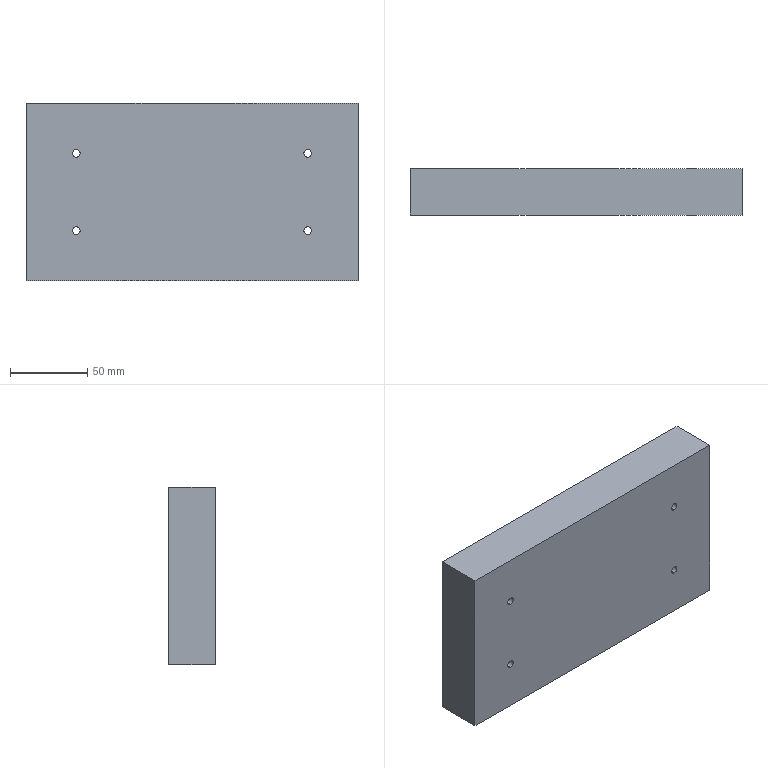Part | SolidWorks | features Extrusion 1, ICE 1 | 1 solid | 14 faces | box 215 x 30 x 115 mm | volume 739394 mm3 | cylinder 8 | plane 6 | commonest cylinder face diameters 5 x8
STEP:
#1=CARTESIAN_POINT('',(-75.,0.,22.5));
#2=VERTEX_POINT('',#1);
#3=CARTESIAN_POINT('',(-75.,0.,27.5));
#4=VERTEX_POINT('',#3);
#5=CARTESIAN_POINT('',(-75.,0.,25.));
#6=DIRECTION('',(0.,1.,0.));
#7=DIRECTION('',(0.,0.,1.));
#8=AXIS2_PLACEMENT_3D('',#5,#6,#7);
#9=CIRCLE('',#8,2.5);
#10=EDGE_CURVE('',#2,#4,#9,.T.);
#11=ORIENTED_EDGE('',*,*,#10,.F.);
#12=CARTESIAN_POINT('',(-75.,30.,22.5));
#13=VERTEX_POINT('',#12);
#14=CARTESIAN_POINT('',(-75.,0.,22.5));
#15=DIRECTION('',(0.,1.,0.));
#16=VECTOR('',#15,1000.);
#17=LINE('',#14,#16);
#18=EDGE_CURVE('',#2,#13,#17,.T.);
#19=ORIENTED_EDGE('',*,*,#18,.T.);
#20=CARTESIAN_POINT('',(-75.,30.,27.5));
#21=VERTEX_POINT('',#20);
#22=CARTESIAN_POINT('',(-75.,30.,25.));
#23=DIRECTION('',(0.,1.,0.));
#24=DIRECTION('',(0.,0.,1.));
#25=AXIS2_PLACEMENT_3D('',#22,#23,#24);
#26=CIRCLE('',#25,2.5);
#27=EDGE_CURVE('',#13,#21,#26,.T.);
#28=ORIENTED_EDGE('',*,*,#27,.T.);
#29=CARTESIAN_POINT('',(-75.,0.,27.5));
#30=DIRECTION('',(0.,1.,0.));
#31=VECTOR('',#30,1000.);
#32=LINE('',#29,#31);
#33=EDGE_CURVE('',#4,#21,#32,.T.);
#34=ORIENTED_EDGE('',*,*,#33,.F.);
#35=EDGE_LOOP('',(#11,#19,#28,#34));
#36=FACE_OUTER_BOUND('',#35,.T.);
#37=CARTESIAN_POINT('',(-75.,0.,25.));
#38=DIRECTION('',(0.,1.,0.));
#39=DIRECTION('',(0.,0.,1.));
#40=AXIS2_PLACEMENT_3D('',#37,#38,#39);
#41=CYLINDRICAL_SURFACE('',#40,2.5);
#42=ADVANCED_FACE('',(#36),#41,.F.);
#43=CARTESIAN_POINT('',(75.,0.,22.5));
#44=VERTEX_POINT('',#43);
#45=CARTESIAN_POINT('',(75.,0.,27.5));
#46=VERTEX_POINT('',#45);
#47=CARTESIAN_POINT('',(75.,0.,25.));
#48=DIRECTION('',(0.,1.,0.));
#49=DIRECTION('',(0.,0.,1.));
#50=AXIS2_PLACEMENT_3D('',#47,#48,#49);
#51=CIRCLE('',#50,2.5);
#52=EDGE_CURVE('',#44,#46,#51,.T.);
#53=ORIENTED_EDGE('',*,*,#52,.F.);
#54=CARTESIAN_POINT('',(75.,30.,22.5));
#55=VERTEX_POINT('',#54);
#56=CARTESIAN_POINT('',(75.,0.,22.5));
#57=DIRECTION('',(0.,1.,0.));
#58=VECTOR('',#57,1000.);
#59=LINE('',#56,#58);
#60=EDGE_CURVE('',#44,#55,#59,.T.);
#61=ORIENTED_EDGE('',*,*,#60,.T.);
#62=CARTESIAN_POINT('',(75.,30.,27.5));
#63=VERTEX_POINT('',#62);
#64=CARTESIAN_POINT('',(75.,30.,25.));
#65=DIRECTION('',(0.,1.,0.));
#66=DIRECTION('',(0.,0.,1.));
#67=AXIS2_PLACEMENT_3D('',#64,#65,#66);
#68=CIRCLE('',#67,2.5);
#69=EDGE_CURVE('',#55,#63,#68,.T.);
#70=ORIENTED_EDGE('',*,*,#69,.T.);
#71=CARTESIAN_POINT('',(75.,0.,27.5));
#72=DIRECTION('',(0.,1.,0.));
#73=VECTOR('',#72,1000.);
#74=LINE('',#71,#73);
#75=EDGE_CURVE('',#46,#63,#74,.T.);
#76=ORIENTED_EDGE('',*,*,#75,.F.);
#77=EDGE_LOOP('',(#53,#61,#70,#76));
#78=FACE_OUTER_BOUND('',#77,.T.);
#79=CARTESIAN_POINT('',(75.,0.,25.));
#80=DIRECTION('',(0.,1.,0.));
#81=DIRECTION('',(0.,0.,1.));
#82=AXIS2_PLACEMENT_3D('',#79,#80,#81);
#83=CYLINDRICAL_SURFACE('',#82,2.5);
#84=ADVANCED_FACE('',(#78),#83,.F.);
#85=CARTESIAN_POINT('',(75.,0.,-27.5));
#86=VERTEX_POINT('',#85);
#87=CARTESIAN_POINT('',(75.,0.,-22.5));
#88=VERTEX_POINT('',#87);
#89=CARTESIAN_POINT('',(75.,0.,-25.));
#90=DIRECTION('',(0.,1.,0.));
#91=DIRECTION('',(0.,0.,1.));
#92=AXIS2_PLACEMENT_3D('',#89,#90,#91);
#93=CIRCLE('',#92,2.5);
#94=EDGE_CURVE('',#86,#88,#93,.T.);
#95=ORIENTED_EDGE('',*,*,#94,.F.);
#96=CARTESIAN_POINT('',(75.,30.,-27.5));
#97=VERTEX_POINT('',#96);
#98=CARTESIAN_POINT('',(75.,0.,-27.5));
#99=DIRECTION('',(0.,1.,0.));
#100=VECTOR('',#99,1000.);
#101=LINE('',#98,#100);
#102=EDGE_CURVE('',#86,#97,#101,.T.);
#103=ORIENTED_EDGE('',*,*,#102,.T.);
#104=CARTESIAN_POINT('',(75.,30.,-22.5));
#105=VERTEX_POINT('',#104);
#106=CARTESIAN_POINT('',(75.,30.,-25.));
#107=DIRECTION('',(0.,1.,0.));
#108=DIRECTION('',(0.,0.,1.));
#109=AXIS2_PLACEMENT_3D('',#106,#107,#108);
#110=CIRCLE('',#109,2.5);
#111=EDGE_CURVE('',#97,#105,#110,.T.);
#112=ORIENTED_EDGE('',*,*,#111,.T.);
#113=CARTESIAN_POINT('',(75.,0.,-22.5));
#114=DIRECTION('',(0.,1.,0.));
#115=VECTOR('',#114,1000.);
#116=LINE('',#113,#115);
#117=EDGE_CURVE('',#88,#105,#116,.T.);
#118=ORIENTED_EDGE('',*,*,#117,.F.);
#119=EDGE_LOOP('',(#95,#103,#112,#118));
#120=FACE_OUTER_BOUND('',#119,.T.);
#121=CARTESIAN_POINT('',(75.,0.,-25.));
#122=DIRECTION('',(0.,1.,0.));
#123=DIRECTION('',(0.,0.,1.));
#124=AXIS2_PLACEMENT_3D('',#121,#122,#123);
#125=CYLINDRICAL_SURFACE('',#124,2.5);
#126=ADVANCED_FACE('',(#120),#125,.F.);
#127=CARTESIAN_POINT('',(-75.,0.,-27.5));
#128=VERTEX_POINT('',#127);
#129=CARTESIAN_POINT('',(-75.,0.,-22.5));
#130=VERTEX_POINT('',#129);
#131=CARTESIAN_POINT('',(-75.,0.,-25.));
#132=DIRECTION('',(0.,1.,0.));
#133=DIRECTION('',(0.,0.,1.));
#134=AXIS2_PLACEMENT_3D('',#131,#132,#133);
#135=CIRCLE('',#134,2.5);
#136=EDGE_CURVE('',#128,#130,#135,.T.);
#137=ORIENTED_EDGE('',*,*,#136,.F.);
#138=CARTESIAN_POINT('',(-75.,30.,-27.5));
#139=VERTEX_POINT('',#138);
#140=CARTESIAN_POINT('',(-75.,0.,-27.5));
#141=DIRECTION('',(0.,1.,0.));
#142=VECTOR('',#141,1000.);
#143=LINE('',#140,#142);
#144=EDGE_CURVE('',#128,#139,#143,.T.);
#145=ORIENTED_EDGE('',*,*,#144,.T.);
#146=CARTESIAN_POINT('',(-75.,30.,-22.5));
#147=VERTEX_POINT('',#146);
#148=CARTESIAN_POINT('',(-75.,30.,-25.));
#149=DIRECTION('',(0.,1.,0.));
#150=DIRECTION('',(0.,0.,1.));
#151=AXIS2_PLACEMENT_3D('',#148,#149,#150);
#152=CIRCLE('',#151,2.5);
#153=EDGE_CURVE('',#139,#147,#152,.T.);
#154=ORIENTED_EDGE('',*,*,#153,.T.);
#155=CARTESIAN_POINT('',(-75.,0.,-22.5));
#156=DIRECTION('',(0.,1.,0.));
#157=VECTOR('',#156,1000.);
#158=LINE('',#155,#157);
#159=EDGE_CURVE('',#130,#147,#158,.T.);
#160=ORIENTED_EDGE('',*,*,#159,.F.);
#161=EDGE_LOOP('',(#137,#145,#154,#160));
#162=FACE_OUTER_BOUND('',#161,.T.);
#163=CARTESIAN_POINT('',(-75.,0.,-25.));
#164=DIRECTION('',(0.,1.,0.));
#165=DIRECTION('',(0.,0.,1.));
#166=AXIS2_PLACEMENT_3D('',#163,#164,#165);
#167=CYLINDRICAL_SURFACE('',#166,2.5);
#168=ADVANCED_FACE('',(#162),#167,.F.);
#169=CARTESIAN_POINT('',(107.5,0.,57.5));
#170=VERTEX_POINT('',#169);
#171=CARTESIAN_POINT('',(107.5,0.,-57.5));
#172=VERTEX_POINT('',#171);
#173=CARTESIAN_POINT('',(107.5,0.,-57.5));
#174=DIRECTION('',(0.,0.,-1.));
#175=VECTOR('',#174,1000.);
#176=LINE('',#173,#175);
#177=EDGE_CURVE('',#170,#172,#176,.T.);
#178=ORIENTED_EDGE('',*,*,#177,.T.);
#179=CARTESIAN_POINT('',(107.5,30.,-57.5));
#180=VERTEX_POINT('',#179);
#181=CARTESIAN_POINT('',(107.5,30.,-57.5));
#182=DIRECTION('',(0.,-1.,0.));
#183=VECTOR('',#182,1000.);
#184=LINE('',#181,#183);
#185=EDGE_CURVE('',#180,#172,#184,.T.);
#186=ORIENTED_EDGE('',*,*,#185,.F.);
#187=CARTESIAN_POINT('',(107.5,30.,57.5));
#188=VERTEX_POINT('',#187);
#189=CARTESIAN_POINT('',(107.5,30.,-57.5));
#190=DIRECTION('',(0.,0.,-1.));
#191=VECTOR('',#190,1000.);
#192=LINE('',#189,#191);
#193=EDGE_CURVE('',#188,#180,#192,.T.);
#194=ORIENTED_EDGE('',*,*,#193,.F.);
#195=CARTESIAN_POINT('',(107.5,30.,57.5));
#196=DIRECTION('',(0.,-1.,0.));
#197=VECTOR('',#196,1000.);
#198=LINE('',#195,#197);
#199=EDGE_CURVE('',#188,#170,#198,.T.);
#200=ORIENTED_EDGE('',*,*,#199,.T.);
#201=EDGE_LOOP('',(#178,#186,#194,#200));
#202=FACE_OUTER_BOUND('',#201,.T.);
#203=CARTESIAN_POINT('',(107.5,30.,-57.5));
#204=DIRECTION('',(-1.,0.,0.));
#205=DIRECTION('',(0.,0.,1.));
#206=AXIS2_PLACEMENT_3D('',#203,#204,#205);
#207=PLANE('',#206);
#208=ADVANCED_FACE('',(#202),#207,.F.);
#209=CARTESIAN_POINT('',(-107.5,0.,-57.5));
#210=VERTEX_POINT('',#209);
#211=CARTESIAN_POINT('',(-107.5,0.,-57.5));
#212=DIRECTION('',(-1.,0.,0.));
#213=VECTOR('',#212,1000.);
#214=LINE('',#211,#213);
#215=EDGE_CURVE('',#172,#210,#214,.T.);
#216=ORIENTED_EDGE('',*,*,#215,.T.);
#217=CARTESIAN_POINT('',(-107.5,30.,-57.5));
#218=VERTEX_POINT('',#217);
#219=CARTESIAN_POINT('',(-107.5,30.,-57.5));
#220=DIRECTION('',(0.,-1.,0.));
#221=VECTOR('',#220,1000.);
#222=LINE('',#219,#221);
#223=EDGE_CURVE('',#218,#210,#222,.T.);
#224=ORIENTED_EDGE('',*,*,#223,.F.);
#225=CARTESIAN_POINT('',(-107.5,30.,-57.5));
#226=DIRECTION('',(-1.,0.,0.));
#227=VECTOR('',#226,1000.);
#228=LINE('',#225,#227);
#229=EDGE_CURVE('',#180,#218,#228,.T.);
#230=ORIENTED_EDGE('',*,*,#229,.F.);
#231=ORIENTED_EDGE('',*,*,#185,.T.);
#232=EDGE_LOOP('',(#216,#224,#230,#231));
#233=FACE_OUTER_BOUND('',#232,.T.);
#234=CARTESIAN_POINT('',(-107.5,30.,-57.5));
#235=DIRECTION('',(0.,0.,1.));
#236=DIRECTION('',(1.,0.,0.));
#237=AXIS2_PLACEMENT_3D('',#234,#235,#236);
#238=PLANE('',#237);
#239=ADVANCED_FACE('',(#233),#238,.F.);
#240=CARTESIAN_POINT('',(-107.5,0.,57.5));
#241=VERTEX_POINT('',#240);
#242=CARTESIAN_POINT('',(-107.5,0.,-57.5));
#243=DIRECTION('',(0.,0.,1.));
#244=VECTOR('',#243,1000.);
#245=LINE('',#242,#244);
#246=EDGE_CURVE('',#210,#241,#245,.T.);
#247=ORIENTED_EDGE('',*,*,#246,.T.);
#248=CARTESIAN_POINT('',(-107.5,30.,57.5));
#249=VERTEX_POINT('',#248);
#250=CARTESIAN_POINT('',(-107.5,30.,57.5));
#251=DIRECTION('',(0.,-1.,0.));
#252=VECTOR('',#251,1000.);
#253=LINE('',#250,#252);
#254=EDGE_CURVE('',#249,#241,#253,.T.);
#255=ORIENTED_EDGE('',*,*,#254,.F.);
#256=CARTESIAN_POINT('',(-107.5,30.,-57.5));
#257=DIRECTION('',(0.,0.,1.));
#258=VECTOR('',#257,1000.);
#259=LINE('',#256,#258);
#260=EDGE_CURVE('',#218,#249,#259,.T.);
#261=ORIENTED_EDGE('',*,*,#260,.F.);
#262=ORIENTED_EDGE('',*,*,#223,.T.);
#263=EDGE_LOOP('',(#247,#255,#261,#262));
#264=FACE_OUTER_BOUND('',#263,.T.);
#265=CARTESIAN_POINT('',(-107.5,30.,-57.5));
#266=DIRECTION('',(1.,0.,0.));
#267=DIRECTION('',(0.,0.,-1.));
#268=AXIS2_PLACEMENT_3D('',#265,#266,#267);
#269=PLANE('',#268);
#270=ADVANCED_FACE('',(#264),#269,.F.);
#271=CARTESIAN_POINT('',(-107.5,0.,57.5));
#272=DIRECTION('',(1.,0.,0.));
#273=VECTOR('',#272,1000.);
#274=LINE('',#271,#273);
#275=EDGE_CURVE('',#241,#170,#274,.T.);
#276=ORIENTED_EDGE('',*,*,#275,.T.);
#277=ORIENTED_EDGE('',*,*,#199,.F.);
#278=CARTESIAN_POINT('',(-107.5,30.,57.5));
#279=DIRECTION('',(1.,0.,0.));
#280=VECTOR('',#279,1000.);
#281=LINE('',#278,#280);
#282=EDGE_CURVE('',#249,#188,#281,.T.);
#283=ORIENTED_EDGE('',*,*,#282,.F.);
#284=ORIENTED_EDGE('',*,*,#254,.T.);
#285=EDGE_LOOP('',(#276,#277,#283,#284));
#286=FACE_OUTER_BOUND('',#285,.T.);
#287=CARTESIAN_POINT('',(-107.5,30.,57.5));
#288=DIRECTION('',(0.,0.,-1.));
#289=DIRECTION('',(-1.,0.,0.));
#290=AXIS2_PLACEMENT_3D('',#287,#288,#289);
#291=PLANE('',#290);
#292=ADVANCED_FACE('',(#286),#291,.F.);
#293=CARTESIAN_POINT('',(-75.,30.,25.));
#294=DIRECTION('',(0.,1.,0.));
#295=DIRECTION('',(0.,0.,1.));
#296=AXIS2_PLACEMENT_3D('',#293,#294,#295);
#297=CIRCLE('',#296,2.5);
#298=EDGE_CURVE('',#21,#13,#297,.T.);
#299=ORIENTED_EDGE('',*,*,#298,.F.);
#300=ORIENTED_EDGE('',*,*,#27,.F.);
#301=EDGE_LOOP('',(#299,#300));
#302=FACE_BOUND('',#301,.T.);
#303=CARTESIAN_POINT('',(75.,30.,25.));
#304=DIRECTION('',(0.,1.,0.));
#305=DIRECTION('',(0.,0.,1.));
#306=AXIS2_PLACEMENT_3D('',#303,#304,#305);
#307=CIRCLE('',#306,2.5);
#308=EDGE_CURVE('',#63,#55,#307,.T.);
#309=ORIENTED_EDGE('',*,*,#308,.F.);
#310=ORIENTED_EDGE('',*,*,#69,.F.);
#311=EDGE_LOOP('',(#309,#310));
#312=FACE_BOUND('',#311,.T.);
#313=CARTESIAN_POINT('',(75.,30.,-25.));
#314=DIRECTION('',(0.,1.,0.));
#315=DIRECTION('',(0.,0.,1.));
#316=AXIS2_PLACEMENT_3D('',#313,#314,#315);
#317=CIRCLE('',#316,2.5);
#318=EDGE_CURVE('',#105,#97,#317,.T.);
#319=ORIENTED_EDGE('',*,*,#318,.F.);
#320=ORIENTED_EDGE('',*,*,#111,.F.);
#321=EDGE_LOOP('',(#319,#320));
#322=FACE_BOUND('',#321,.T.);
#323=CARTESIAN_POINT('',(-75.,30.,-25.));
#324=DIRECTION('',(0.,1.,0.));
#325=DIRECTION('',(0.,0.,1.));
#326=AXIS2_PLACEMENT_3D('',#323,#324,#325);
#327=CIRCLE('',#326,2.5);
#328=EDGE_CURVE('',#147,#139,#327,.T.);
#329=ORIENTED_EDGE('',*,*,#328,.F.);
#330=ORIENTED_EDGE('',*,*,#153,.F.);
#331=EDGE_LOOP('',(#329,#330));
#332=FACE_BOUND('',#331,.T.);
#333=ORIENTED_EDGE('',*,*,#193,.T.);
#334=ORIENTED_EDGE('',*,*,#229,.T.);
#335=ORIENTED_EDGE('',*,*,#260,.T.);
#336=ORIENTED_EDGE('',*,*,#282,.T.);
#337=EDGE_LOOP('',(#333,#334,#335,#336));
#338=FACE_OUTER_BOUND('',#337,.T.);
#339=CARTESIAN_POINT('',(0.,30.,0.));
#340=DIRECTION('',(0.,1.,0.));
#341=DIRECTION('',(0.,0.,1.));
#342=AXIS2_PLACEMENT_3D('',#339,#340,#341);
#343=PLANE('',#342);
#344=ADVANCED_FACE('',(#302,#312,#322,#332,#338),#343,.T.);
#345=CARTESIAN_POINT('',(-75.,0.,25.));
#346=DIRECTION('',(0.,1.,0.));
#347=DIRECTION('',(0.,0.,1.));
#348=AXIS2_PLACEMENT_3D('',#345,#346,#347);
#349=CIRCLE('',#348,2.5);
#350=EDGE_CURVE('',#4,#2,#349,.T.);
#351=ORIENTED_EDGE('',*,*,#350,.T.);
#352=ORIENTED_EDGE('',*,*,#10,.T.);
#353=EDGE_LOOP('',(#351,#352));
#354=FACE_BOUND('',#353,.T.);
#355=CARTESIAN_POINT('',(75.,0.,25.));
#356=DIRECTION('',(0.,1.,0.));
#357=DIRECTION('',(0.,0.,1.));
#358=AXIS2_PLACEMENT_3D('',#355,#356,#357);
#359=CIRCLE('',#358,2.5);
#360=EDGE_CURVE('',#46,#44,#359,.T.);
#361=ORIENTED_EDGE('',*,*,#360,.T.);
#362=ORIENTED_EDGE('',*,*,#52,.T.);
#363=EDGE_LOOP('',(#361,#362));
#364=FACE_BOUND('',#363,.T.);
#365=CARTESIAN_POINT('',(75.,0.,-25.));
#366=DIRECTION('',(0.,1.,0.));
#367=DIRECTION('',(0.,0.,1.));
#368=AXIS2_PLACEMENT_3D('',#365,#366,#367);
#369=CIRCLE('',#368,2.5);
#370=EDGE_CURVE('',#88,#86,#369,.T.);
#371=ORIENTED_EDGE('',*,*,#370,.T.);
#372=ORIENTED_EDGE('',*,*,#94,.T.);
#373=EDGE_LOOP('',(#371,#372));
#374=FACE_BOUND('',#373,.T.);
#375=CARTESIAN_POINT('',(-75.,0.,-25.));
#376=DIRECTION('',(0.,1.,0.));
#377=DIRECTION('',(0.,0.,1.));
#378=AXIS2_PLACEMENT_3D('',#375,#376,#377);
#379=CIRCLE('',#378,2.5);
#380=EDGE_CURVE('',#130,#128,#379,.T.);
#381=ORIENTED_EDGE('',*,*,#380,.T.);
#382=ORIENTED_EDGE('',*,*,#136,.T.);
#383=EDGE_LOOP('',(#381,#382));
#384=FACE_BOUND('',#383,.T.);
#385=ORIENTED_EDGE('',*,*,#177,.F.);
#386=ORIENTED_EDGE('',*,*,#275,.F.);
#387=ORIENTED_EDGE('',*,*,#246,.F.);
#388=ORIENTED_EDGE('',*,*,#215,.F.);
#389=EDGE_LOOP('',(#385,#386,#387,#388));
#390=FACE_OUTER_BOUND('',#389,.T.);
#391=CARTESIAN_POINT('',(0.,0.,0.));
#392=DIRECTION('',(0.,1.,0.));
#393=DIRECTION('',(0.,0.,1.));
#394=AXIS2_PLACEMENT_3D('',#391,#392,#393);
#395=PLANE('',#394);
#396=ADVANCED_FACE('',(#354,#364,#374,#384,#390),#395,.F.);
#397=ORIENTED_EDGE('',*,*,#144,.F.);
#398=ORIENTED_EDGE('',*,*,#380,.F.);
#399=ORIENTED_EDGE('',*,*,#159,.T.);
#400=ORIENTED_EDGE('',*,*,#328,.T.);
#401=EDGE_LOOP('',(#397,#398,#399,#400));
#402=FACE_OUTER_BOUND('',#401,.T.);
#403=CARTESIAN_POINT('',(-75.,0.,-25.));
#404=DIRECTION('',(0.,1.,0.));
#405=DIRECTION('',(0.,0.,1.));
#406=AXIS2_PLACEMENT_3D('',#403,#404,#405);
#407=CYLINDRICAL_SURFACE('',#406,2.5);
#408=ADVANCED_FACE('',(#402),#407,.F.);
#409=ORIENTED_EDGE('',*,*,#102,.F.);
#410=ORIENTED_EDGE('',*,*,#370,.F.);
#411=ORIENTED_EDGE('',*,*,#117,.T.);
#412=ORIENTED_EDGE('',*,*,#318,.T.);
#413=EDGE_LOOP('',(#409,#410,#411,#412));
#414=FACE_OUTER_BOUND('',#413,.T.);
#415=CARTESIAN_POINT('',(75.,0.,-25.));
#416=DIRECTION('',(0.,1.,0.));
#417=DIRECTION('',(0.,0.,1.));
#418=AXIS2_PLACEMENT_3D('',#415,#416,#417);
#419=CYLINDRICAL_SURFACE('',#418,2.5);
#420=ADVANCED_FACE('',(#414),#419,.F.);
#421=ORIENTED_EDGE('',*,*,#60,.F.);
#422=ORIENTED_EDGE('',*,*,#360,.F.);
#423=ORIENTED_EDGE('',*,*,#75,.T.);
#424=ORIENTED_EDGE('',*,*,#308,.T.);
#425=EDGE_LOOP('',(#421,#422,#423,#424));
#426=FACE_OUTER_BOUND('',#425,.T.);
#427=CARTESIAN_POINT('',(75.,0.,25.));
#428=DIRECTION('',(0.,1.,0.));
#429=DIRECTION('',(0.,0.,1.));
#430=AXIS2_PLACEMENT_3D('',#427,#428,#429);
#431=CYLINDRICAL_SURFACE('',#430,2.5);
#432=ADVANCED_FACE('',(#426),#431,.F.);
#433=ORIENTED_EDGE('',*,*,#18,.F.);
#434=ORIENTED_EDGE('',*,*,#350,.F.);
#435=ORIENTED_EDGE('',*,*,#33,.T.);
#436=ORIENTED_EDGE('',*,*,#298,.T.);
#437=EDGE_LOOP('',(#433,#434,#435,#436));
#438=FACE_OUTER_BOUND('',#437,.T.);
#439=CARTESIAN_POINT('',(-75.,0.,25.));
#440=DIRECTION('',(0.,1.,0.));
#441=DIRECTION('',(0.,0.,1.));
#442=AXIS2_PLACEMENT_3D('',#439,#440,#441);
#443=CYLINDRICAL_SURFACE('',#442,2.5);
#444=ADVANCED_FACE('',(#438),#443,.F.);
#445=CLOSED_SHELL('',(#42,#84,#126,#168,#208,#239,#270,#292,#344,#396,#408,#420,#432,#444));
#446=MANIFOLD_SOLID_BREP('',#445);
#447=CARTESIAN_POINT('',(0.,0.,0.));
#448=DIRECTION('',(0.,0.,1.));
#449=DIRECTION('',(1.,0.,0.));
#450=AXIS2_PLACEMENT_3D('',#447,#448,#449);
#451=(LENGTH_UNIT()NAMED_UNIT(*)SI_UNIT(.MILLI.,.METRE.));
#452=UNCERTAINTY_MEASURE_WITH_UNIT(LENGTH_MEASURE(0.00001),#451,'','');
#453=(NAMED_UNIT(*)PLANE_ANGLE_UNIT()SI_UNIT($,.RADIAN.));
#454=(NAMED_UNIT(*)SI_UNIT($,.STERADIAN.)SOLID_ANGLE_UNIT());
#455=(GEOMETRIC_REPRESENTATION_CONTEXT(3)GLOBAL_UNCERTAINTY_ASSIGNED_CONTEXT((#452))GLOBAL_UNIT_ASSIGNED_CONTEXT((#451,#453,#454))REPRESENTATION_CONTEXT('',''));
#456=ADVANCED_BREP_SHAPE_REPRESENTATION('',(#446,#450),#455);